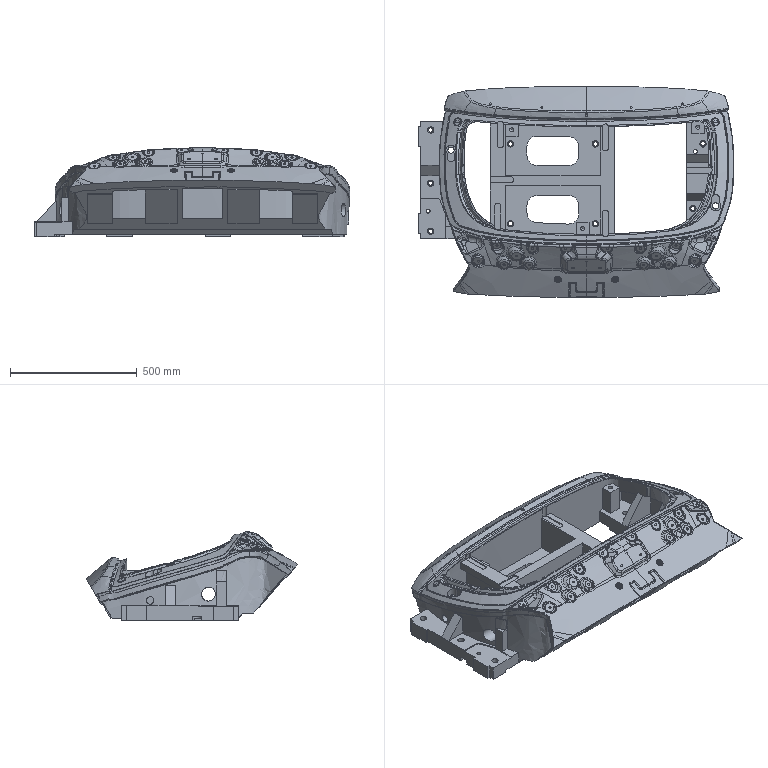Part | NX | features solid 2 | 1 solid | 1320 faces | box 1247 x 834.126 x 352.916 mm | volume 93635382 mm3 | spline 1018 | plane 229 | cylinder 70 | cone 3 | commonest cylinder face diameters 20 x14 25 x13 17 x9 80 x8 27 x7 16 x5